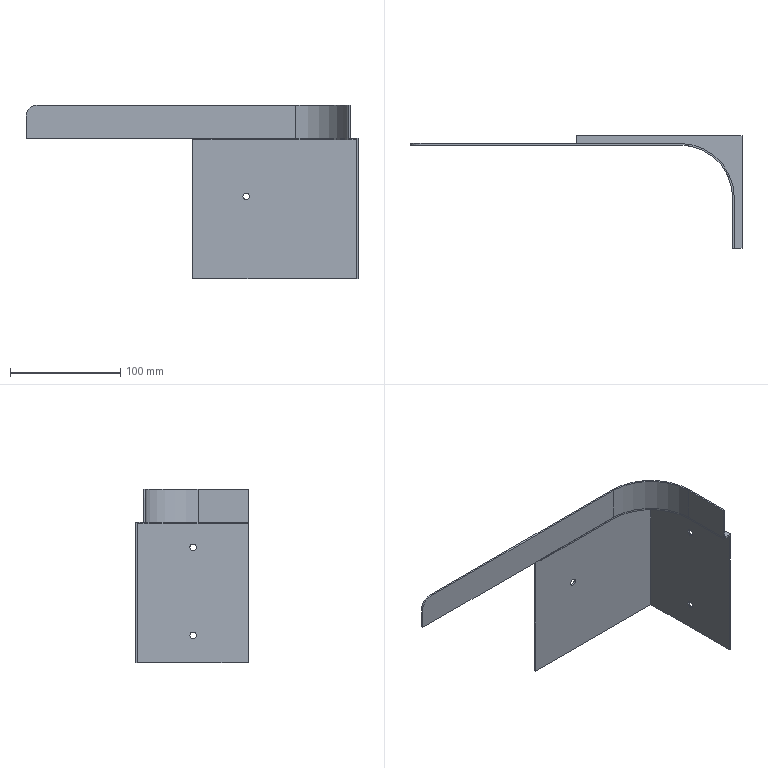Part | STEP file | 2 solids | 29 faces | box 301.5 x 102 x 158 mm | volume 67738 mm3 | plane 19 | cylinder 10 | commonest cylinder face diameters 6 x6 96 x2 20 x1 99 x1